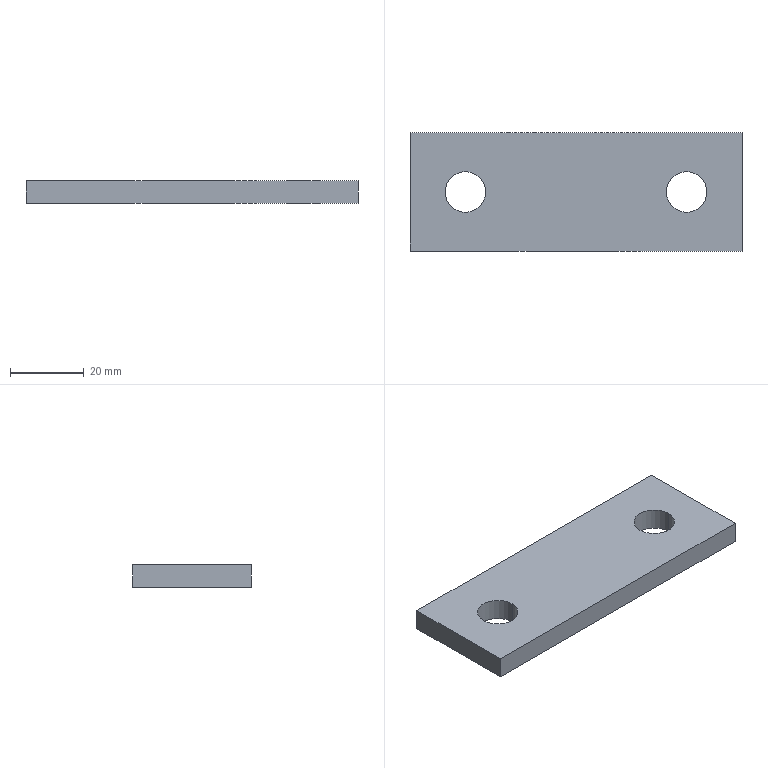Part | SolidWorks | features Extrusion 1, ICE 1, LPattern 1 | 1 solid | 10 faces | box 90 x 32 x 6 mm | volume 16140 mm3 | plane 6 | cylinder 4 | commonest cylinder face diameters 11 x4
STEP:
#1=CARTESIAN_POINT('',(69.5,-16.,0.));
#2=VERTEX_POINT('',#1);
#3=CARTESIAN_POINT('',(80.5,-16.,0.));
#4=VERTEX_POINT('',#3);
#5=CARTESIAN_POINT('',(75.,-16.,0.));
#6=DIRECTION('',(0.,0.,1.));
#7=DIRECTION('',(1.,0.,0.));
#8=AXIS2_PLACEMENT_3D('',#5,#6,#7);
#9=CIRCLE('',#8,5.5);
#10=EDGE_CURVE('',#2,#4,#9,.T.);
#11=ORIENTED_EDGE('',*,*,#10,.F.);
#12=CARTESIAN_POINT('',(69.5,-16.,6.));
#13=VERTEX_POINT('',#12);
#14=CARTESIAN_POINT('',(69.5,-16.,0.));
#15=DIRECTION('',(0.,0.,1.));
#16=VECTOR('',#15,1000.);
#17=LINE('',#14,#16);
#18=EDGE_CURVE('',#2,#13,#17,.T.);
#19=ORIENTED_EDGE('',*,*,#18,.T.);
#20=CARTESIAN_POINT('',(80.5,-16.,6.));
#21=VERTEX_POINT('',#20);
#22=CARTESIAN_POINT('',(75.,-16.,6.));
#23=DIRECTION('',(0.,0.,1.));
#24=DIRECTION('',(1.,0.,0.));
#25=AXIS2_PLACEMENT_3D('',#22,#23,#24);
#26=CIRCLE('',#25,5.5);
#27=EDGE_CURVE('',#13,#21,#26,.T.);
#28=ORIENTED_EDGE('',*,*,#27,.T.);
#29=CARTESIAN_POINT('',(80.5,-16.,0.));
#30=DIRECTION('',(0.,0.,1.));
#31=VECTOR('',#30,1000.);
#32=LINE('',#29,#31);
#33=EDGE_CURVE('',#4,#21,#32,.T.);
#34=ORIENTED_EDGE('',*,*,#33,.F.);
#35=EDGE_LOOP('',(#11,#19,#28,#34));
#36=FACE_OUTER_BOUND('',#35,.T.);
#37=CARTESIAN_POINT('',(75.,-16.,0.));
#38=DIRECTION('',(0.,0.,1.));
#39=DIRECTION('',(1.,0.,0.));
#40=AXIS2_PLACEMENT_3D('',#37,#38,#39);
#41=CYLINDRICAL_SURFACE('',#40,5.5);
#42=ADVANCED_FACE('',(#36),#41,.F.);
#43=CARTESIAN_POINT('',(9.5,-16.,0.));
#44=VERTEX_POINT('',#43);
#45=CARTESIAN_POINT('',(20.5,-16.,0.));
#46=VERTEX_POINT('',#45);
#47=CARTESIAN_POINT('',(15.,-16.,0.));
#48=DIRECTION('',(0.,0.,1.));
#49=DIRECTION('',(1.,0.,0.));
#50=AXIS2_PLACEMENT_3D('',#47,#48,#49);
#51=CIRCLE('',#50,5.5);
#52=EDGE_CURVE('',#44,#46,#51,.T.);
#53=ORIENTED_EDGE('',*,*,#52,.F.);
#54=CARTESIAN_POINT('',(9.5,-16.,6.));
#55=VERTEX_POINT('',#54);
#56=CARTESIAN_POINT('',(9.5,-16.,0.));
#57=DIRECTION('',(0.,0.,1.));
#58=VECTOR('',#57,1000.);
#59=LINE('',#56,#58);
#60=EDGE_CURVE('',#44,#55,#59,.T.);
#61=ORIENTED_EDGE('',*,*,#60,.T.);
#62=CARTESIAN_POINT('',(20.5,-16.,6.));
#63=VERTEX_POINT('',#62);
#64=CARTESIAN_POINT('',(15.,-16.,6.));
#65=DIRECTION('',(0.,0.,1.));
#66=DIRECTION('',(1.,0.,0.));
#67=AXIS2_PLACEMENT_3D('',#64,#65,#66);
#68=CIRCLE('',#67,5.5);
#69=EDGE_CURVE('',#55,#63,#68,.T.);
#70=ORIENTED_EDGE('',*,*,#69,.T.);
#71=CARTESIAN_POINT('',(20.5,-16.,0.));
#72=DIRECTION('',(0.,0.,1.));
#73=VECTOR('',#72,1000.);
#74=LINE('',#71,#73);
#75=EDGE_CURVE('',#46,#63,#74,.T.);
#76=ORIENTED_EDGE('',*,*,#75,.F.);
#77=EDGE_LOOP('',(#53,#61,#70,#76));
#78=FACE_OUTER_BOUND('',#77,.T.);
#79=CARTESIAN_POINT('',(15.,-16.,0.));
#80=DIRECTION('',(0.,0.,1.));
#81=DIRECTION('',(1.,0.,0.));
#82=AXIS2_PLACEMENT_3D('',#79,#80,#81);
#83=CYLINDRICAL_SURFACE('',#82,5.5);
#84=ADVANCED_FACE('',(#78),#83,.F.);
#85=CARTESIAN_POINT('',(90.,-32.,0.));
#86=VERTEX_POINT('',#85);
#87=CARTESIAN_POINT('',(90.,0.,0.));
#88=VERTEX_POINT('',#87);
#89=CARTESIAN_POINT('',(90.,0.,0.));
#90=DIRECTION('',(0.,1.,0.));
#91=VECTOR('',#90,1000.);
#92=LINE('',#89,#91);
#93=EDGE_CURVE('',#86,#88,#92,.T.);
#94=ORIENTED_EDGE('',*,*,#93,.T.);
#95=CARTESIAN_POINT('',(90.,0.,6.));
#96=VERTEX_POINT('',#95);
#97=CARTESIAN_POINT('',(90.,0.,6.));
#98=DIRECTION('',(0.,0.,-1.));
#99=VECTOR('',#98,1000.);
#100=LINE('',#97,#99);
#101=EDGE_CURVE('',#96,#88,#100,.T.);
#102=ORIENTED_EDGE('',*,*,#101,.F.);
#103=CARTESIAN_POINT('',(90.,-32.,6.));
#104=VERTEX_POINT('',#103);
#105=CARTESIAN_POINT('',(90.,0.,6.));
#106=DIRECTION('',(0.,1.,0.));
#107=VECTOR('',#106,1000.);
#108=LINE('',#105,#107);
#109=EDGE_CURVE('',#104,#96,#108,.T.);
#110=ORIENTED_EDGE('',*,*,#109,.F.);
#111=CARTESIAN_POINT('',(90.,-32.,6.));
#112=DIRECTION('',(0.,0.,-1.));
#113=VECTOR('',#112,1000.);
#114=LINE('',#111,#113);
#115=EDGE_CURVE('',#104,#86,#114,.T.);
#116=ORIENTED_EDGE('',*,*,#115,.T.);
#117=EDGE_LOOP('',(#94,#102,#110,#116));
#118=FACE_OUTER_BOUND('',#117,.T.);
#119=CARTESIAN_POINT('',(90.,0.,6.));
#120=DIRECTION('',(-1.,0.,0.));
#121=DIRECTION('',(0.,0.,1.));
#122=AXIS2_PLACEMENT_3D('',#119,#120,#121);
#123=PLANE('',#122);
#124=ADVANCED_FACE('',(#118),#123,.F.);
#125=CARTESIAN_POINT('',(0.,0.,0.));
#126=VERTEX_POINT('',#125);
#127=CARTESIAN_POINT('',(0.,0.,0.));
#128=DIRECTION('',(-1.,0.,0.));
#129=VECTOR('',#128,1000.);
#130=LINE('',#127,#129);
#131=EDGE_CURVE('',#88,#126,#130,.T.);
#132=ORIENTED_EDGE('',*,*,#131,.T.);
#133=CARTESIAN_POINT('',(0.,0.,6.));
#134=VERTEX_POINT('',#133);
#135=CARTESIAN_POINT('',(0.,0.,6.));
#136=DIRECTION('',(0.,0.,-1.));
#137=VECTOR('',#136,1000.);
#138=LINE('',#135,#137);
#139=EDGE_CURVE('',#134,#126,#138,.T.);
#140=ORIENTED_EDGE('',*,*,#139,.F.);
#141=CARTESIAN_POINT('',(0.,0.,6.));
#142=DIRECTION('',(-1.,0.,0.));
#143=VECTOR('',#142,1000.);
#144=LINE('',#141,#143);
#145=EDGE_CURVE('',#96,#134,#144,.T.);
#146=ORIENTED_EDGE('',*,*,#145,.F.);
#147=ORIENTED_EDGE('',*,*,#101,.T.);
#148=EDGE_LOOP('',(#132,#140,#146,#147));
#149=FACE_OUTER_BOUND('',#148,.T.);
#150=CARTESIAN_POINT('',(0.,0.,6.));
#151=DIRECTION('',(0.,-1.,0.));
#152=DIRECTION('',(0.,0.,-1.));
#153=AXIS2_PLACEMENT_3D('',#150,#151,#152);
#154=PLANE('',#153);
#155=ADVANCED_FACE('',(#149),#154,.F.);
#156=CARTESIAN_POINT('',(0.,-32.,0.));
#157=VERTEX_POINT('',#156);
#158=CARTESIAN_POINT('',(0.,0.,0.));
#159=DIRECTION('',(0.,-1.,0.));
#160=VECTOR('',#159,1000.);
#161=LINE('',#158,#160);
#162=EDGE_CURVE('',#126,#157,#161,.T.);
#163=ORIENTED_EDGE('',*,*,#162,.T.);
#164=CARTESIAN_POINT('',(0.,-32.,6.));
#165=VERTEX_POINT('',#164);
#166=CARTESIAN_POINT('',(0.,-32.,6.));
#167=DIRECTION('',(0.,0.,-1.));
#168=VECTOR('',#167,1000.);
#169=LINE('',#166,#168);
#170=EDGE_CURVE('',#165,#157,#169,.T.);
#171=ORIENTED_EDGE('',*,*,#170,.F.);
#172=CARTESIAN_POINT('',(0.,0.,6.));
#173=DIRECTION('',(0.,-1.,0.));
#174=VECTOR('',#173,1000.);
#175=LINE('',#172,#174);
#176=EDGE_CURVE('',#134,#165,#175,.T.);
#177=ORIENTED_EDGE('',*,*,#176,.F.);
#178=ORIENTED_EDGE('',*,*,#139,.T.);
#179=EDGE_LOOP('',(#163,#171,#177,#178));
#180=FACE_OUTER_BOUND('',#179,.T.);
#181=CARTESIAN_POINT('',(0.,0.,6.));
#182=DIRECTION('',(1.,0.,0.));
#183=DIRECTION('',(0.,1.,0.));
#184=AXIS2_PLACEMENT_3D('',#181,#182,#183);
#185=PLANE('',#184);
#186=ADVANCED_FACE('',(#180),#185,.F.);
#187=CARTESIAN_POINT('',(0.,-32.,0.));
#188=DIRECTION('',(1.,0.,0.));
#189=VECTOR('',#188,1000.);
#190=LINE('',#187,#189);
#191=EDGE_CURVE('',#157,#86,#190,.T.);
#192=ORIENTED_EDGE('',*,*,#191,.T.);
#193=ORIENTED_EDGE('',*,*,#115,.F.);
#194=CARTESIAN_POINT('',(0.,-32.,6.));
#195=DIRECTION('',(1.,0.,0.));
#196=VECTOR('',#195,1000.);
#197=LINE('',#194,#196);
#198=EDGE_CURVE('',#165,#104,#197,.T.);
#199=ORIENTED_EDGE('',*,*,#198,.F.);
#200=ORIENTED_EDGE('',*,*,#170,.T.);
#201=EDGE_LOOP('',(#192,#193,#199,#200));
#202=FACE_OUTER_BOUND('',#201,.T.);
#203=CARTESIAN_POINT('',(0.,-32.,6.));
#204=DIRECTION('',(0.,1.,0.));
#205=DIRECTION('',(0.,0.,1.));
#206=AXIS2_PLACEMENT_3D('',#203,#204,#205);
#207=PLANE('',#206);
#208=ADVANCED_FACE('',(#202),#207,.F.);
#209=CARTESIAN_POINT('',(75.,-16.,6.));
#210=DIRECTION('',(0.,0.,1.));
#211=DIRECTION('',(1.,0.,0.));
#212=AXIS2_PLACEMENT_3D('',#209,#210,#211);
#213=CIRCLE('',#212,5.5);
#214=EDGE_CURVE('',#21,#13,#213,.T.);
#215=ORIENTED_EDGE('',*,*,#214,.F.);
#216=ORIENTED_EDGE('',*,*,#27,.F.);
#217=EDGE_LOOP('',(#215,#216));
#218=FACE_BOUND('',#217,.T.);
#219=CARTESIAN_POINT('',(15.,-16.,6.));
#220=DIRECTION('',(0.,0.,1.));
#221=DIRECTION('',(1.,0.,0.));
#222=AXIS2_PLACEMENT_3D('',#219,#220,#221);
#223=CIRCLE('',#222,5.5);
#224=EDGE_CURVE('',#63,#55,#223,.T.);
#225=ORIENTED_EDGE('',*,*,#224,.F.);
#226=ORIENTED_EDGE('',*,*,#69,.F.);
#227=EDGE_LOOP('',(#225,#226));
#228=FACE_BOUND('',#227,.T.);
#229=ORIENTED_EDGE('',*,*,#109,.T.);
#230=ORIENTED_EDGE('',*,*,#145,.T.);
#231=ORIENTED_EDGE('',*,*,#176,.T.);
#232=ORIENTED_EDGE('',*,*,#198,.T.);
#233=EDGE_LOOP('',(#229,#230,#231,#232));
#234=FACE_OUTER_BOUND('',#233,.T.);
#235=CARTESIAN_POINT('',(0.,0.,6.));
#236=DIRECTION('',(0.,0.,1.));
#237=DIRECTION('',(1.,0.,0.));
#238=AXIS2_PLACEMENT_3D('',#235,#236,#237);
#239=PLANE('',#238);
#240=ADVANCED_FACE('',(#218,#228,#234),#239,.T.);
#241=CARTESIAN_POINT('',(75.,-16.,0.));
#242=DIRECTION('',(0.,0.,1.));
#243=DIRECTION('',(1.,0.,0.));
#244=AXIS2_PLACEMENT_3D('',#241,#242,#243);
#245=CIRCLE('',#244,5.5);
#246=EDGE_CURVE('',#4,#2,#245,.T.);
#247=ORIENTED_EDGE('',*,*,#246,.T.);
#248=ORIENTED_EDGE('',*,*,#10,.T.);
#249=EDGE_LOOP('',(#247,#248));
#250=FACE_BOUND('',#249,.T.);
#251=CARTESIAN_POINT('',(15.,-16.,0.));
#252=DIRECTION('',(0.,0.,1.));
#253=DIRECTION('',(1.,0.,0.));
#254=AXIS2_PLACEMENT_3D('',#251,#252,#253);
#255=CIRCLE('',#254,5.5);
#256=EDGE_CURVE('',#46,#44,#255,.T.);
#257=ORIENTED_EDGE('',*,*,#256,.T.);
#258=ORIENTED_EDGE('',*,*,#52,.T.);
#259=EDGE_LOOP('',(#257,#258));
#260=FACE_BOUND('',#259,.T.);
#261=ORIENTED_EDGE('',*,*,#93,.F.);
#262=ORIENTED_EDGE('',*,*,#191,.F.);
#263=ORIENTED_EDGE('',*,*,#162,.F.);
#264=ORIENTED_EDGE('',*,*,#131,.F.);
#265=EDGE_LOOP('',(#261,#262,#263,#264));
#266=FACE_OUTER_BOUND('',#265,.T.);
#267=CARTESIAN_POINT('',(0.,0.,0.));
#268=DIRECTION('',(0.,0.,1.));
#269=DIRECTION('',(1.,0.,0.));
#270=AXIS2_PLACEMENT_3D('',#267,#268,#269);
#271=PLANE('',#270);
#272=ADVANCED_FACE('',(#250,#260,#266),#271,.F.);
#273=ORIENTED_EDGE('',*,*,#60,.F.);
#274=ORIENTED_EDGE('',*,*,#256,.F.);
#275=ORIENTED_EDGE('',*,*,#75,.T.);
#276=ORIENTED_EDGE('',*,*,#224,.T.);
#277=EDGE_LOOP('',(#273,#274,#275,#276));
#278=FACE_OUTER_BOUND('',#277,.T.);
#279=CARTESIAN_POINT('',(15.,-16.,0.));
#280=DIRECTION('',(0.,0.,1.));
#281=DIRECTION('',(1.,0.,0.));
#282=AXIS2_PLACEMENT_3D('',#279,#280,#281);
#283=CYLINDRICAL_SURFACE('',#282,5.5);
#284=ADVANCED_FACE('',(#278),#283,.F.);
#285=ORIENTED_EDGE('',*,*,#18,.F.);
#286=ORIENTED_EDGE('',*,*,#246,.F.);
#287=ORIENTED_EDGE('',*,*,#33,.T.);
#288=ORIENTED_EDGE('',*,*,#214,.T.);
#289=EDGE_LOOP('',(#285,#286,#287,#288));
#290=FACE_OUTER_BOUND('',#289,.T.);
#291=CARTESIAN_POINT('',(75.,-16.,0.));
#292=DIRECTION('',(0.,0.,1.));
#293=DIRECTION('',(1.,0.,0.));
#294=AXIS2_PLACEMENT_3D('',#291,#292,#293);
#295=CYLINDRICAL_SURFACE('',#294,5.5);
#296=ADVANCED_FACE('',(#290),#295,.F.);
#297=CLOSED_SHELL('',(#42,#84,#124,#155,#186,#208,#240,#272,#284,#296));
#298=MANIFOLD_SOLID_BREP('',#297);
#299=CARTESIAN_POINT('',(0.,0.,0.));
#300=DIRECTION('',(0.,0.,1.));
#301=DIRECTION('',(1.,0.,0.));
#302=AXIS2_PLACEMENT_3D('',#299,#300,#301);
#303=(LENGTH_UNIT()NAMED_UNIT(*)SI_UNIT(.MILLI.,.METRE.));
#304=UNCERTAINTY_MEASURE_WITH_UNIT(LENGTH_MEASURE(0.00001),#303,'','');
#305=(NAMED_UNIT(*)PLANE_ANGLE_UNIT()SI_UNIT($,.RADIAN.));
#306=(NAMED_UNIT(*)SI_UNIT($,.STERADIAN.)SOLID_ANGLE_UNIT());
#307=(GEOMETRIC_REPRESENTATION_CONTEXT(3)GLOBAL_UNCERTAINTY_ASSIGNED_CONTEXT((#304))GLOBAL_UNIT_ASSIGNED_CONTEXT((#303,#305,#306))REPRESENTATION_CONTEXT('',''));
#308=ADVANCED_BREP_SHAPE_REPRESENTATION('',(#298,#302),#307);